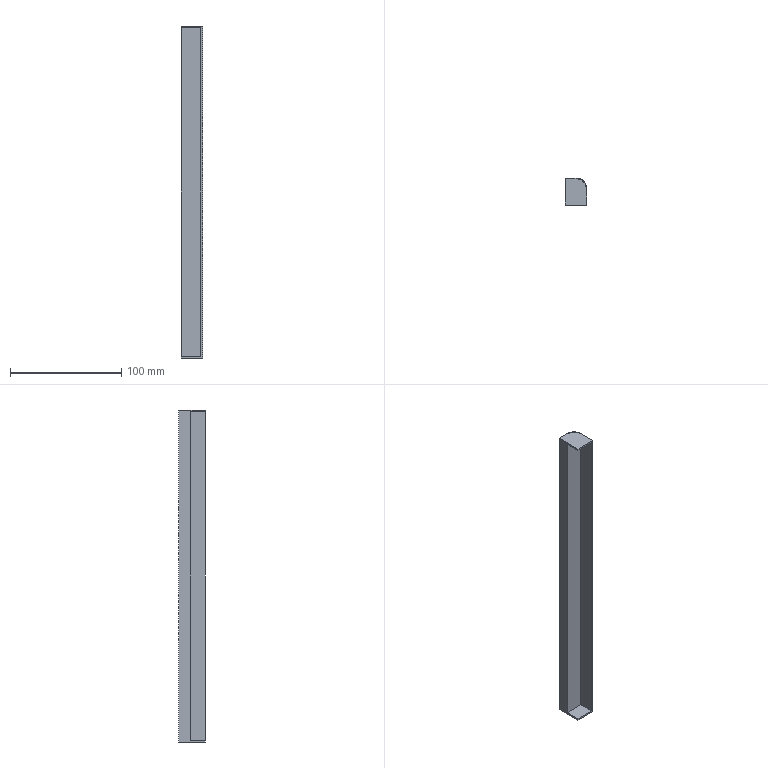Part | SolidWorks | features BaseBody 1 | 1 solid | 25 faces | box 19 x 24 x 298 mm | volume 61282 mm3 | cylinder 15 | plane 10 | commonest cylinder face diameters 1 x8 18 x7
STEP:
#1=CARTESIAN_POINT('',(17.2,0.,295.));
#2=VERTEX_POINT('',#1);
#3=CARTESIAN_POINT('',(17.2,0.,0.));
#4=VERTEX_POINT('',#3);
#5=CARTESIAN_POINT('',(17.2,0.,295.));
#6=DIRECTION('',(0.,0.,-1.));
#7=VECTOR('',#6,1000.);
#8=LINE('',#5,#7);
#9=EDGE_CURVE('',#2,#4,#8,.T.);
#10=ORIENTED_EDGE('',*,*,#9,.F.);
#11=CARTESIAN_POINT('',(0.,0.,295.));
#12=VERTEX_POINT('',#11);
#13=CARTESIAN_POINT('',(0.,0.,295.));
#14=DIRECTION('',(1.,0.,0.));
#15=VECTOR('',#14,1000.);
#16=LINE('',#13,#15);
#17=EDGE_CURVE('',#12,#2,#16,.T.);
#18=ORIENTED_EDGE('',*,*,#17,.F.);
#19=CARTESIAN_POINT('',(0.,0.,0.));
#20=VERTEX_POINT('',#19);
#21=CARTESIAN_POINT('',(0.,0.,295.));
#22=DIRECTION('',(0.,0.,1.));
#23=VECTOR('',#22,1000.);
#24=LINE('',#21,#23);
#25=EDGE_CURVE('',#20,#12,#24,.T.);
#26=ORIENTED_EDGE('',*,*,#25,.F.);
#27=CARTESIAN_POINT('',(0.,0.,0.));
#28=DIRECTION('',(-1.,0.,0.));
#29=VECTOR('',#28,1000.);
#30=LINE('',#27,#29);
#31=EDGE_CURVE('',#4,#20,#30,.T.);
#32=ORIENTED_EDGE('',*,*,#31,.F.);
#33=EDGE_LOOP('',(#10,#18,#26,#32));
#34=FACE_OUTER_BOUND('',#33,.T.);
#35=CARTESIAN_POINT('',(0.,0.,295.));
#36=DIRECTION('',(0.,1.,0.));
#37=DIRECTION('',(0.,0.,1.));
#38=AXIS2_PLACEMENT_3D('',#35,#36,#37);
#39=PLANE('',#38);
#40=ADVANCED_FACE('',(#34),#39,.F.);
#41=CARTESIAN_POINT('',(0.,-13.5,0.));
#42=VERTEX_POINT('',#41);
#43=CARTESIAN_POINT('',(0.,1.5,0.));
#44=DIRECTION('',(0.,1.,0.));
#45=VECTOR('',#44,1000.);
#46=LINE('',#43,#45);
#47=EDGE_CURVE('',#42,#20,#46,.T.);
#48=ORIENTED_EDGE('',*,*,#47,.F.);
#49=CARTESIAN_POINT('',(17.2,-13.5,0.));
#50=VERTEX_POINT('',#49);
#51=CARTESIAN_POINT('',(10.,-13.5,0.));
#52=DIRECTION('',(-1.,0.,0.));
#53=VECTOR('',#52,1000.);
#54=LINE('',#51,#53);
#55=EDGE_CURVE('',#50,#42,#54,.T.);
#56=ORIENTED_EDGE('',*,*,#55,.F.);
#57=CARTESIAN_POINT('',(17.2,1.5,0.));
#58=DIRECTION('',(0.,-1.,0.));
#59=VECTOR('',#58,1000.);
#60=LINE('',#57,#59);
#61=EDGE_CURVE('',#4,#50,#60,.T.);
#62=ORIENTED_EDGE('',*,*,#61,.F.);
#63=ORIENTED_EDGE('',*,*,#31,.T.);
#64=EDGE_LOOP('',(#48,#56,#62,#63));
#65=FACE_OUTER_BOUND('',#64,.T.);
#66=CARTESIAN_POINT('',(10.,1.5,0.));
#67=DIRECTION('',(0.,0.,-1.));
#68=DIRECTION('',(-1.,0.,0.));
#69=AXIS2_PLACEMENT_3D('',#66,#67,#68);
#70=PLANE('',#69);
#71=ADVANCED_FACE('',(#65),#70,.F.);
#72=CARTESIAN_POINT('',(17.2,-13.5,295.));
#73=VERTEX_POINT('',#72);
#74=CARTESIAN_POINT('',(17.2,-13.5,295.));
#75=DIRECTION('',(0.,0.,-1.));
#76=VECTOR('',#75,1000.);
#77=LINE('',#74,#76);
#78=EDGE_CURVE('',#73,#50,#77,.T.);
#79=ORIENTED_EDGE('',*,*,#78,.F.);
#80=CARTESIAN_POINT('',(17.2,0.,295.));
#81=DIRECTION('',(0.,-1.,0.));
#82=VECTOR('',#81,1000.);
#83=LINE('',#80,#82);
#84=EDGE_CURVE('',#2,#73,#83,.T.);
#85=ORIENTED_EDGE('',*,*,#84,.F.);
#86=ORIENTED_EDGE('',*,*,#9,.T.);
#87=ORIENTED_EDGE('',*,*,#61,.T.);
#88=EDGE_LOOP('',(#79,#85,#86,#87));
#89=FACE_OUTER_BOUND('',#88,.T.);
#90=CARTESIAN_POINT('',(17.2,0.,295.));
#91=DIRECTION('',(1.,0.,0.));
#92=DIRECTION('',(0.,0.,-1.));
#93=AXIS2_PLACEMENT_3D('',#90,#91,#92);
#94=PLANE('',#93);
#95=ADVANCED_FACE('',(#89),#94,.F.);
#96=ORIENTED_EDGE('',*,*,#17,.T.);
#97=ORIENTED_EDGE('',*,*,#84,.T.);
#98=CARTESIAN_POINT('',(0.,-13.5,295.));
#99=VERTEX_POINT('',#98);
#100=CARTESIAN_POINT('',(10.,-13.5,295.));
#101=DIRECTION('',(1.,0.,0.));
#102=VECTOR('',#101,1000.);
#103=LINE('',#100,#102);
#104=EDGE_CURVE('',#99,#73,#103,.T.);
#105=ORIENTED_EDGE('',*,*,#104,.F.);
#106=CARTESIAN_POINT('',(0.,1.5,295.));
#107=DIRECTION('',(0.,-1.,0.));
#108=VECTOR('',#107,1000.);
#109=LINE('',#106,#108);
#110=EDGE_CURVE('',#12,#99,#109,.T.);
#111=ORIENTED_EDGE('',*,*,#110,.F.);
#112=EDGE_LOOP('',(#96,#97,#105,#111));
#113=FACE_OUTER_BOUND('',#112,.T.);
#114=CARTESIAN_POINT('',(10.,1.5,295.));
#115=DIRECTION('',(0.,0.,1.));
#116=DIRECTION('',(1.,0.,0.));
#117=AXIS2_PLACEMENT_3D('',#114,#115,#116);
#118=PLANE('',#117);
#119=ADVANCED_FACE('',(#113),#118,.F.);
#120=CARTESIAN_POINT('',(0.,-13.5,-1.5));
#121=VERTEX_POINT('',#120);
#122=CARTESIAN_POINT('',(0.,10.5,-1.5));
#123=VERTEX_POINT('',#122);
#124=CARTESIAN_POINT('',(0.,0.,-1.5));
#125=DIRECTION('',(0.,1.,0.));
#126=VECTOR('',#125,1000.);
#127=LINE('',#124,#126);
#128=EDGE_CURVE('',#121,#123,#127,.T.);
#129=ORIENTED_EDGE('',*,*,#128,.F.);
#130=CARTESIAN_POINT('',(0.,-13.5,295.));
#131=DIRECTION('',(0.,0.,-1.));
#132=VECTOR('',#131,1000.);
#133=LINE('',#130,#132);
#134=EDGE_CURVE('',#42,#121,#133,.T.);
#135=ORIENTED_EDGE('',*,*,#134,.F.);
#136=ORIENTED_EDGE('',*,*,#47,.T.);
#137=ORIENTED_EDGE('',*,*,#25,.T.);
#138=ORIENTED_EDGE('',*,*,#110,.T.);
#139=CARTESIAN_POINT('',(0.,-13.5,296.5));
#140=VERTEX_POINT('',#139);
#141=CARTESIAN_POINT('',(0.,-13.5,295.));
#142=DIRECTION('',(0.,0.,-1.));
#143=VECTOR('',#142,1000.);
#144=LINE('',#141,#143);
#145=EDGE_CURVE('',#140,#99,#144,.T.);
#146=ORIENTED_EDGE('',*,*,#145,.F.);
#147=CARTESIAN_POINT('',(0.,10.5,296.5));
#148=VERTEX_POINT('',#147);
#149=CARTESIAN_POINT('',(0.,0.,296.5));
#150=DIRECTION('',(0.,-1.,0.));
#151=VECTOR('',#150,1000.);
#152=LINE('',#149,#151);
#153=EDGE_CURVE('',#148,#140,#152,.T.);
#154=ORIENTED_EDGE('',*,*,#153,.F.);
#155=CARTESIAN_POINT('',(0.,10.5,295.));
#156=DIRECTION('',(0.,0.,1.));
#157=VECTOR('',#156,1000.);
#158=LINE('',#155,#157);
#159=EDGE_CURVE('',#123,#148,#158,.T.);
#160=ORIENTED_EDGE('',*,*,#159,.F.);
#161=EDGE_LOOP('',(#129,#135,#136,#137,#138,#146,#154,#160));
#162=FACE_OUTER_BOUND('',#161,.T.);
#163=CARTESIAN_POINT('',(0.,0.,295.));
#164=DIRECTION('',(1.,0.,0.));
#165=DIRECTION('',(0.,0.,-1.));
#166=AXIS2_PLACEMENT_3D('',#163,#164,#165);
#167=PLANE('',#166);
#168=ADVANCED_FACE('',(#162),#167,.F.);
#169=ORIENTED_EDGE('',*,*,#55,.T.);
#170=ORIENTED_EDGE('',*,*,#134,.T.);
#171=CARTESIAN_POINT('',(19.,-13.5,-1.5));
#172=VERTEX_POINT('',#171);
#173=CARTESIAN_POINT('',(17.2,-13.5,-1.5));
#174=DIRECTION('',(-1.,0.,0.));
#175=VECTOR('',#174,1000.);
#176=LINE('',#173,#175);
#177=EDGE_CURVE('',#172,#121,#176,.T.);
#178=ORIENTED_EDGE('',*,*,#177,.F.);
#179=CARTESIAN_POINT('',(19.,-13.5,296.5));
#180=VERTEX_POINT('',#179);
#181=CARTESIAN_POINT('',(19.,-13.5,295.));
#182=DIRECTION('',(0.,0.,-1.));
#183=VECTOR('',#182,1000.);
#184=LINE('',#181,#183);
#185=EDGE_CURVE('',#180,#172,#184,.T.);
#186=ORIENTED_EDGE('',*,*,#185,.F.);
#187=CARTESIAN_POINT('',(17.2,-13.5,296.5));
#188=DIRECTION('',(1.,0.,0.));
#189=VECTOR('',#188,1000.);
#190=LINE('',#187,#189);
#191=EDGE_CURVE('',#140,#180,#190,.T.);
#192=ORIENTED_EDGE('',*,*,#191,.F.);
#193=ORIENTED_EDGE('',*,*,#145,.T.);
#194=ORIENTED_EDGE('',*,*,#104,.T.);
#195=ORIENTED_EDGE('',*,*,#78,.T.);
#196=EDGE_LOOP('',(#169,#170,#178,#186,#192,#193,#194,#195));
#197=FACE_OUTER_BOUND('',#196,.T.);
#198=CARTESIAN_POINT('',(17.2,-13.5,295.));
#199=DIRECTION('',(0.,1.,0.));
#200=DIRECTION('',(0.,0.,1.));
#201=AXIS2_PLACEMENT_3D('',#198,#199,#200);
#202=PLANE('',#201);
#203=ADVANCED_FACE('',(#197),#202,.F.);
#204=CARTESIAN_POINT('',(9.5,10.5,-1.5));
#205=VERTEX_POINT('',#204);
#206=CARTESIAN_POINT('',(9.5,10.5,296.5));
#207=VERTEX_POINT('',#206);
#208=CARTESIAN_POINT('',(9.5,10.5,295.));
#209=DIRECTION('',(0.,0.,1.));
#210=VECTOR('',#209,1000.);
#211=LINE('',#208,#210);
#212=EDGE_CURVE('',#205,#207,#211,.T.);
#213=ORIENTED_EDGE('',*,*,#212,.F.);
#214=CARTESIAN_POINT('',(0.,10.5,-1.5));
#215=DIRECTION('',(1.,0.,0.));
#216=VECTOR('',#215,1000.);
#217=LINE('',#214,#216);
#218=EDGE_CURVE('',#123,#205,#217,.T.);
#219=ORIENTED_EDGE('',*,*,#218,.F.);
#220=ORIENTED_EDGE('',*,*,#159,.T.);
#221=CARTESIAN_POINT('',(0.,10.5,296.5));
#222=DIRECTION('',(-1.,0.,0.));
#223=VECTOR('',#222,1000.);
#224=LINE('',#221,#223);
#225=EDGE_CURVE('',#207,#148,#224,.T.);
#226=ORIENTED_EDGE('',*,*,#225,.F.);
#227=EDGE_LOOP('',(#213,#219,#220,#226));
#228=FACE_OUTER_BOUND('',#227,.T.);
#229=CARTESIAN_POINT('',(0.,10.5,295.));
#230=DIRECTION('',(0.,-1.,0.));
#231=DIRECTION('',(0.,0.,-1.));
#232=AXIS2_PLACEMENT_3D('',#229,#230,#231);
#233=PLANE('',#232);
#234=ADVANCED_FACE('',(#228),#233,.F.);
#235=ORIENTED_EDGE('',*,*,#128,.T.);
#236=ORIENTED_EDGE('',*,*,#218,.T.);
#237=CARTESIAN_POINT('',(10.5,10.486,-1.5));
#238=VERTEX_POINT('',#237);
#239=CARTESIAN_POINT('',(10.,10.5,-1.5));
#240=DIRECTION('',(0.,0.,1.));
#241=DIRECTION('',(1.,0.,0.));
#242=AXIS2_PLACEMENT_3D('',#239,#240,#241);
#243=CIRCLE('',#242,0.5);
#244=EDGE_CURVE('',#205,#238,#243,.T.);
#245=ORIENTED_EDGE('',*,*,#244,.T.);
#246=CARTESIAN_POINT('',(11.512,10.372,-1.5));
#247=VERTEX_POINT('',#246);
#248=CARTESIAN_POINT('',(10.,1.5,-1.5));
#249=DIRECTION('',(0.,0.,1.));
#250=DIRECTION('',(-1.,0.,0.));
#251=AXIS2_PLACEMENT_3D('',#248,#249,#250);
#252=CIRCLE('',#251,9.);
#253=EDGE_CURVE('',#247,#238,#252,.T.);
#254=ORIENTED_EDGE('',*,*,#253,.F.);
#255=CARTESIAN_POINT('',(12.487,10.15,-1.5));
#256=VERTEX_POINT('',#255);
#257=CARTESIAN_POINT('',(12.003,10.274,-1.5));
#258=DIRECTION('',(0.,0.,1.));
#259=DIRECTION('',(1.,0.,0.));
#260=AXIS2_PLACEMENT_3D('',#257,#258,#259);
#261=CIRCLE('',#260,0.5);
#262=EDGE_CURVE('',#247,#256,#261,.T.);
#263=ORIENTED_EDGE('',*,*,#262,.T.);
#264=CARTESIAN_POINT('',(13.449,9.813,-1.5));
#265=VERTEX_POINT('',#264);
#266=CARTESIAN_POINT('',(10.,1.5,-1.5));
#267=DIRECTION('',(0.,0.,1.));
#268=DIRECTION('',(-1.,0.,0.));
#269=AXIS2_PLACEMENT_3D('',#266,#267,#268);
#270=CIRCLE('',#269,9.);
#271=EDGE_CURVE('',#265,#256,#270,.T.);
#272=ORIENTED_EDGE('',*,*,#271,.F.);
#273=CARTESIAN_POINT('',(14.349,9.379,-1.5));
#274=VERTEX_POINT('',#273);
#275=CARTESIAN_POINT('',(13.905,9.609,-1.5));
#276=DIRECTION('',(0.,0.,1.));
#277=DIRECTION('',(1.,0.,0.));
#278=AXIS2_PLACEMENT_3D('',#275,#276,#277);
#279=CIRCLE('',#278,0.5);
#280=EDGE_CURVE('',#265,#274,#279,.T.);
#281=ORIENTED_EDGE('',*,*,#280,.T.);
#282=CARTESIAN_POINT('',(15.212,8.837,-1.5));
#283=VERTEX_POINT('',#282);
#284=CARTESIAN_POINT('',(10.,1.5,-1.5));
#285=DIRECTION('',(0.,0.,1.));
#286=DIRECTION('',(-1.,0.,0.));
#287=AXIS2_PLACEMENT_3D('',#284,#285,#286);
#288=CIRCLE('',#287,9.);
#289=EDGE_CURVE('',#283,#274,#288,.T.);
#290=ORIENTED_EDGE('',*,*,#289,.F.);
#291=CARTESIAN_POINT('',(15.994,8.214,-1.5));
#292=VERTEX_POINT('',#291);
#293=CARTESIAN_POINT('',(15.611,8.536,-1.5));
#294=DIRECTION('',(0.,0.,1.));
#295=DIRECTION('',(1.,0.,0.));
#296=AXIS2_PLACEMENT_3D('',#293,#294,#295);
#297=CIRCLE('',#296,0.5);
#298=EDGE_CURVE('',#283,#292,#297,.T.);
#299=ORIENTED_EDGE('',*,*,#298,.T.);
#300=CARTESIAN_POINT('',(16.714,7.494,-1.5));
#301=VERTEX_POINT('',#300);
#302=CARTESIAN_POINT('',(10.,1.5,-1.5));
#303=DIRECTION('',(0.,0.,1.));
#304=DIRECTION('',(-1.,0.,0.));
#305=AXIS2_PLACEMENT_3D('',#302,#303,#304);
#306=CIRCLE('',#305,9.);
#307=EDGE_CURVE('',#301,#292,#306,.T.);
#308=ORIENTED_EDGE('',*,*,#307,.F.);
#309=CARTESIAN_POINT('',(17.337,6.712,-1.5));
#310=VERTEX_POINT('',#309);
#311=CARTESIAN_POINT('',(17.036,7.111,-1.5));
#312=DIRECTION('',(0.,0.,1.));
#313=DIRECTION('',(1.,0.,0.));
#314=AXIS2_PLACEMENT_3D('',#311,#312,#313);
#315=CIRCLE('',#314,0.5);
#316=EDGE_CURVE('',#301,#310,#315,.T.);
#317=ORIENTED_EDGE('',*,*,#316,.T.);
#318=CARTESIAN_POINT('',(17.879,5.849,-1.5));
#319=VERTEX_POINT('',#318);
#320=CARTESIAN_POINT('',(10.,1.5,-1.5));
#321=DIRECTION('',(0.,0.,1.));
#322=DIRECTION('',(-1.,0.,0.));
#323=AXIS2_PLACEMENT_3D('',#320,#321,#322);
#324=CIRCLE('',#323,9.);
#325=EDGE_CURVE('',#319,#310,#324,.T.);
#326=ORIENTED_EDGE('',*,*,#325,.F.);
#327=CARTESIAN_POINT('',(18.313,4.949,-1.5));
#328=VERTEX_POINT('',#327);
#329=CARTESIAN_POINT('',(18.109,5.405,-1.5));
#330=DIRECTION('',(0.,0.,1.));
#331=DIRECTION('',(1.,0.,0.));
#332=AXIS2_PLACEMENT_3D('',#329,#330,#331);
#333=CIRCLE('',#332,0.5);
#334=EDGE_CURVE('',#319,#328,#333,.T.);
#335=ORIENTED_EDGE('',*,*,#334,.T.);
#336=CARTESIAN_POINT('',(18.65,3.987,-1.5));
#337=VERTEX_POINT('',#336);
#338=CARTESIAN_POINT('',(10.,1.5,-1.5));
#339=DIRECTION('',(0.,0.,1.));
#340=DIRECTION('',(-1.,0.,0.));
#341=AXIS2_PLACEMENT_3D('',#338,#339,#340);
#342=CIRCLE('',#341,9.);
#343=EDGE_CURVE('',#337,#328,#342,.T.);
#344=ORIENTED_EDGE('',*,*,#343,.F.);
#345=CARTESIAN_POINT('',(18.872,3.012,-1.5));
#346=VERTEX_POINT('',#345);
#347=CARTESIAN_POINT('',(18.774,3.503,-1.5));
#348=DIRECTION('',(0.,0.,1.));
#349=DIRECTION('',(1.,0.,0.));
#350=AXIS2_PLACEMENT_3D('',#347,#348,#349);
#351=CIRCLE('',#350,0.5);
#352=EDGE_CURVE('',#337,#346,#351,.T.);
#353=ORIENTED_EDGE('',*,*,#352,.T.);
#354=CARTESIAN_POINT('',(18.986,2.,-1.5));
#355=VERTEX_POINT('',#354);
#356=CARTESIAN_POINT('',(10.,1.5,-1.5));
#357=DIRECTION('',(0.,0.,1.));
#358=DIRECTION('',(-1.,0.,0.));
#359=AXIS2_PLACEMENT_3D('',#356,#357,#358);
#360=CIRCLE('',#359,9.);
#361=EDGE_CURVE('',#355,#346,#360,.T.);
#362=ORIENTED_EDGE('',*,*,#361,.F.);
#363=CARTESIAN_POINT('',(19.,1.,-1.5));
#364=VERTEX_POINT('',#363);
#365=CARTESIAN_POINT('',(19.,1.5,-1.5));
#366=DIRECTION('',(0.,0.,1.));
#367=DIRECTION('',(1.,0.,0.));
#368=AXIS2_PLACEMENT_3D('',#365,#366,#367);
#369=CIRCLE('',#368,0.5);
#370=EDGE_CURVE('',#355,#364,#369,.T.);
#371=ORIENTED_EDGE('',*,*,#370,.T.);
#372=CARTESIAN_POINT('',(19.,1.5,-1.5));
#373=DIRECTION('',(0.,-1.,0.));
#374=VECTOR('',#373,1000.);
#375=LINE('',#372,#374);
#376=EDGE_CURVE('',#364,#172,#375,.T.);
#377=ORIENTED_EDGE('',*,*,#376,.T.);
#378=ORIENTED_EDGE('',*,*,#177,.T.);
#379=EDGE_LOOP('',(#235,#236,#245,#254,#263,#272,#281,#290,#299,#308,#317,#326,#335,#344,#353,#362,#371,#377,#378));
#380=FACE_OUTER_BOUND('',#379,.T.);
#381=CARTESIAN_POINT('',(10.,1.5,-1.5));
#382=DIRECTION('',(0.,0.,-1.));
#383=DIRECTION('',(-1.,0.,0.));
#384=AXIS2_PLACEMENT_3D('',#381,#382,#383);
#385=PLANE('',#384);
#386=ADVANCED_FACE('',(#380),#385,.T.);
#387=CARTESIAN_POINT('',(12.487,10.15,296.5));
#388=VERTEX_POINT('',#387);
#389=CARTESIAN_POINT('',(11.512,10.372,296.5));
#390=VERTEX_POINT('',#389);
#391=CARTESIAN_POINT('',(12.003,10.274,296.5));
#392=DIRECTION('',(0.,0.,-1.));
#393=DIRECTION('',(1.,0.,0.));
#394=AXIS2_PLACEMENT_3D('',#391,#392,#393);
#395=CIRCLE('',#394,0.5);
#396=EDGE_CURVE('',#388,#390,#395,.T.);
#397=ORIENTED_EDGE('',*,*,#396,.T.);
#398=CARTESIAN_POINT('',(10.5,10.486,296.5));
#399=VERTEX_POINT('',#398);
#400=CARTESIAN_POINT('',(10.,1.5,296.5));
#401=DIRECTION('',(0.,0.,-1.));
#402=DIRECTION('',(-1.,0.,0.));
#403=AXIS2_PLACEMENT_3D('',#400,#401,#402);
#404=CIRCLE('',#403,9.);
#405=EDGE_CURVE('',#399,#390,#404,.T.);
#406=ORIENTED_EDGE('',*,*,#405,.F.);
#407=CARTESIAN_POINT('',(10.,10.5,296.5));
#408=DIRECTION('',(0.,0.,-1.));
#409=DIRECTION('',(1.,0.,0.));
#410=AXIS2_PLACEMENT_3D('',#407,#408,#409);
#411=CIRCLE('',#410,0.5);
#412=EDGE_CURVE('',#399,#207,#411,.T.);
#413=ORIENTED_EDGE('',*,*,#412,.T.);
#414=ORIENTED_EDGE('',*,*,#225,.T.);
#415=ORIENTED_EDGE('',*,*,#153,.T.);
#416=ORIENTED_EDGE('',*,*,#191,.T.);
#417=CARTESIAN_POINT('',(19.,1.,296.5));
#418=VERTEX_POINT('',#417);
#419=CARTESIAN_POINT('',(19.,1.5,296.5));
#420=DIRECTION('',(0.,1.,0.));
#421=VECTOR('',#420,1000.);
#422=LINE('',#419,#421);
#423=EDGE_CURVE('',#180,#418,#422,.T.);
#424=ORIENTED_EDGE('',*,*,#423,.T.);
#425=CARTESIAN_POINT('',(18.986,2.,296.5));
#426=VERTEX_POINT('',#425);
#427=CARTESIAN_POINT('',(19.,1.5,296.5));
#428=DIRECTION('',(0.,0.,-1.));
#429=DIRECTION('',(1.,0.,0.));
#430=AXIS2_PLACEMENT_3D('',#427,#428,#429);
#431=CIRCLE('',#430,0.5);
#432=EDGE_CURVE('',#418,#426,#431,.T.);
#433=ORIENTED_EDGE('',*,*,#432,.T.);
#434=CARTESIAN_POINT('',(18.872,3.012,296.5));
#435=VERTEX_POINT('',#434);
#436=CARTESIAN_POINT('',(10.,1.5,296.5));
#437=DIRECTION('',(0.,0.,-1.));
#438=DIRECTION('',(-1.,0.,0.));
#439=AXIS2_PLACEMENT_3D('',#436,#437,#438);
#440=CIRCLE('',#439,9.);
#441=EDGE_CURVE('',#435,#426,#440,.T.);
#442=ORIENTED_EDGE('',*,*,#441,.F.);
#443=CARTESIAN_POINT('',(18.65,3.987,296.5));
#444=VERTEX_POINT('',#443);
#445=CARTESIAN_POINT('',(18.774,3.503,296.5));
#446=DIRECTION('',(0.,0.,-1.));
#447=DIRECTION('',(1.,0.,0.));
#448=AXIS2_PLACEMENT_3D('',#445,#446,#447);
#449=CIRCLE('',#448,0.5);
#450=EDGE_CURVE('',#435,#444,#449,.T.);
#451=ORIENTED_EDGE('',*,*,#450,.T.);
#452=CARTESIAN_POINT('',(18.313,4.949,296.5));
#453=VERTEX_POINT('',#452);
#454=CARTESIAN_POINT('',(10.,1.5,296.5));
#455=DIRECTION('',(0.,0.,-1.));
#456=DIRECTION('',(-1.,0.,0.));
#457=AXIS2_PLACEMENT_3D('',#454,#455,#456);
#458=CIRCLE('',#457,9.);
#459=EDGE_CURVE('',#453,#444,#458,.T.);
#460=ORIENTED_EDGE('',*,*,#459,.F.);
#461=CARTESIAN_POINT('',(17.879,5.849,296.5));
#462=VERTEX_POINT('',#461);
#463=CARTESIAN_POINT('',(18.109,5.405,296.5));
#464=DIRECTION('',(0.,0.,-1.));
#465=DIRECTION('',(1.,0.,0.));
#466=AXIS2_PLACEMENT_3D('',#463,#464,#465);
#467=CIRCLE('',#466,0.5);
#468=EDGE_CURVE('',#453,#462,#467,.T.);
#469=ORIENTED_EDGE('',*,*,#468,.T.);
#470=CARTESIAN_POINT('',(17.337,6.712,296.5));
#471=VERTEX_POINT('',#470);
#472=CARTESIAN_POINT('',(10.,1.5,296.5));
#473=DIRECTION('',(0.,0.,-1.));
#474=DIRECTION('',(-1.,0.,0.));
#475=AXIS2_PLACEMENT_3D('',#472,#473,#474);
#476=CIRCLE('',#475,9.);
#477=EDGE_CURVE('',#471,#462,#476,.T.);
#478=ORIENTED_EDGE('',*,*,#477,.F.);
#479=CARTESIAN_POINT('',(16.714,7.494,296.5));
#480=VERTEX_POINT('',#479);
#481=CARTESIAN_POINT('',(17.036,7.111,296.5));
#482=DIRECTION('',(0.,0.,-1.));
#483=DIRECTION('',(1.,0.,0.));
#484=AXIS2_PLACEMENT_3D('',#481,#482,#483);
#485=CIRCLE('',#484,0.5);
#486=EDGE_CURVE('',#471,#480,#485,.T.);
#487=ORIENTED_EDGE('',*,*,#486,.T.);
#488=CARTESIAN_POINT('',(15.994,8.214,296.5));
#489=VERTEX_POINT('',#488);
#490=CARTESIAN_POINT('',(10.,1.5,296.5));
#491=DIRECTION('',(0.,0.,-1.));
#492=DIRECTION('',(-1.,0.,0.));
#493=AXIS2_PLACEMENT_3D('',#490,#491,#492);
#494=CIRCLE('',#493,9.);
#495=EDGE_CURVE('',#489,#480,#494,.T.);
#496=ORIENTED_EDGE('',*,*,#495,.F.);
#497=CARTESIAN_POINT('',(15.212,8.837,296.5));
#498=VERTEX_POINT('',#497);
#499=CARTESIAN_POINT('',(15.611,8.536,296.5));
#500=DIRECTION('',(0.,0.,-1.));
#501=DIRECTION('',(1.,0.,0.));
#502=AXIS2_PLACEMENT_3D('',#499,#500,#501);
#503=CIRCLE('',#502,0.5);
#504=EDGE_CURVE('',#489,#498,#503,.T.);
#505=ORIENTED_EDGE('',*,*,#504,.T.);
#506=CARTESIAN_POINT('',(14.349,9.379,296.5));
#507=VERTEX_POINT('',#506);
#508=CARTESIAN_POINT('',(10.,1.5,296.5));
#509=DIRECTION('',(0.,0.,-1.));
#510=DIRECTION('',(-1.,0.,0.));
#511=AXIS2_PLACEMENT_3D('',#508,#509,#510);
#512=CIRCLE('',#511,9.);
#513=EDGE_CURVE('',#507,#498,#512,.T.);
#514=ORIENTED_EDGE('',*,*,#513,.F.);
#515=CARTESIAN_POINT('',(13.449,9.813,296.5));
#516=VERTEX_POINT('',#515);
#517=CARTESIAN_POINT('',(13.905,9.609,296.5));
#518=DIRECTION('',(0.,0.,-1.));
#519=DIRECTION('',(1.,0.,0.));
#520=AXIS2_PLACEMENT_3D('',#517,#518,#519);
#521=CIRCLE('',#520,0.5);
#522=EDGE_CURVE('',#507,#516,#521,.T.);
#523=ORIENTED_EDGE('',*,*,#522,.T.);
#524=CARTESIAN_POINT('',(10.,1.5,296.5));
#525=DIRECTION('',(0.,0.,-1.));
#526=DIRECTION('',(-1.,0.,0.));
#527=AXIS2_PLACEMENT_3D('',#524,#525,#526);
#528=CIRCLE('',#527,9.);
#529=EDGE_CURVE('',#388,#516,#528,.T.);
#530=ORIENTED_EDGE('',*,*,#529,.F.);
#531=EDGE_LOOP('',(#397,#406,#413,#414,#415,#416,#424,#433,#442,#451,#460,#469,#478,#487,#496,#505,#514,#523,#530));
#532=FACE_OUTER_BOUND('',#531,.T.);
#533=CARTESIAN_POINT('',(10.,1.5,296.5));
#534=DIRECTION('',(0.,0.,1.));
#535=DIRECTION('',(1.,0.,0.));
#536=AXIS2_PLACEMENT_3D('',#533,#534,#535);
#537=PLANE('',#536);
#538=ADVANCED_FACE('',(#532),#537,.T.);
#539=CARTESIAN_POINT('',(19.,1.,295.));
#540=DIRECTION('',(0.,0.,-1.));
#541=VECTOR('',#540,1000.);
#542=LINE('',#539,#541);
#543=EDGE_CURVE('',#418,#364,#542,.T.);
#544=ORIENTED_EDGE('',*,*,#543,.F.);
#545=ORIENTED_EDGE('',*,*,#423,.F.);
#546=ORIENTED_EDGE('',*,*,#185,.T.);
#547=ORIENTED_EDGE('',*,*,#376,.F.);
#548=EDGE_LOOP('',(#544,#545,#546,#547));
#549=FACE_OUTER_BOUND('',#548,.T.);
#550=CARTESIAN_POINT('',(19.,1.5,295.));
#551=DIRECTION('',(-1.,0.,0.));
#552=DIRECTION('',(0.,-1.,0.));
#553=AXIS2_PLACEMENT_3D('',#550,#551,#552);
#554=PLANE('',#553);
#555=ADVANCED_FACE('',(#549),#554,.F.);
#556=ORIENTED_EDGE('',*,*,#212,.T.);
#557=ORIENTED_EDGE('',*,*,#412,.F.);
#558=CARTESIAN_POINT('',(10.5,10.486,-1.5));
#559=DIRECTION('',(0.,0.,1.));
#560=VECTOR('',#559,1000.);
#561=LINE('',#558,#560);
#562=EDGE_CURVE('',#238,#399,#561,.T.);
#563=ORIENTED_EDGE('',*,*,#562,.F.);
#564=ORIENTED_EDGE('',*,*,#244,.F.);
#565=EDGE_LOOP('',(#556,#557,#563,#564));
#566=FACE_OUTER_BOUND('',#565,.T.);
#567=CARTESIAN_POINT('',(10.,10.5,-1.5));
#568=DIRECTION('',(0.,0.,1.));
#569=DIRECTION('',(1.,0.,0.));
#570=AXIS2_PLACEMENT_3D('',#567,#568,#569);
#571=CYLINDRICAL_SURFACE('',#570,0.5);
#572=ADVANCED_FACE('',(#566),#571,.F.);
#573=CARTESIAN_POINT('',(18.986,2.,-1.5));
#574=DIRECTION('',(0.,0.,-1.));
#575=VECTOR('',#574,1000.);
#576=LINE('',#573,#575);
#577=EDGE_CURVE('',#426,#355,#576,.T.);
#578=ORIENTED_EDGE('',*,*,#577,.F.);
#579=ORIENTED_EDGE('',*,*,#432,.F.);
#580=ORIENTED_EDGE('',*,*,#543,.T.);
#581=ORIENTED_EDGE('',*,*,#370,.F.);
#582=EDGE_LOOP('',(#578,#579,#580,#581));
#583=FACE_OUTER_BOUND('',#582,.T.);
#584=CARTESIAN_POINT('',(19.,1.5,-1.5));
#585=DIRECTION('',(0.,0.,1.));
#586=DIRECTION('',(1.,0.,0.));
#587=AXIS2_PLACEMENT_3D('',#584,#585,#586);
#588=CYLINDRICAL_SURFACE('',#587,0.5);
#589=ADVANCED_FACE('',(#583),#588,.F.);
#590=ORIENTED_EDGE('',*,*,#405,.T.);
#591=CARTESIAN_POINT('',(11.512,10.372,295.));
#592=DIRECTION('',(0.,0.,-1.));
#593=VECTOR('',#592,1000.);
#594=LINE('',#591,#593);
#595=EDGE_CURVE('',#390,#247,#594,.T.);
#596=ORIENTED_EDGE('',*,*,#595,.T.);
#597=ORIENTED_EDGE('',*,*,#253,.T.);
#598=ORIENTED_EDGE('',*,*,#562,.T.);
#599=EDGE_LOOP('',(#590,#596,#597,#598));
#600=FACE_OUTER_BOUND('',#599,.T.);
#601=CARTESIAN_POINT('',(10.,1.5,295.));
#602=DIRECTION('',(0.,0.,-1.));
#603=DIRECTION('',(-1.,0.,0.));
#604=AXIS2_PLACEMENT_3D('',#601,#602,#603);
#605=CYLINDRICAL_SURFACE('',#604,9.);
#606=ADVANCED_FACE('',(#600),#605,.T.);
#607=ORIENTED_EDGE('',*,*,#441,.T.);
#608=ORIENTED_EDGE('',*,*,#577,.T.);
#609=ORIENTED_EDGE('',*,*,#361,.T.);
#610=CARTESIAN_POINT('',(18.872,3.012,295.));
#611=DIRECTION('',(0.,0.,1.));
#612=VECTOR('',#611,1000.);
#613=LINE('',#610,#612);
#614=EDGE_CURVE('',#346,#435,#613,.T.);
#615=ORIENTED_EDGE('',*,*,#614,.T.);
#616=EDGE_LOOP('',(#607,#608,#609,#615));
#617=FACE_OUTER_BOUND('',#616,.T.);
#618=CARTESIAN_POINT('',(10.,1.5,295.));
#619=DIRECTION('',(0.,0.,-1.));
#620=DIRECTION('',(-1.,0.,0.));
#621=AXIS2_PLACEMENT_3D('',#618,#619,#620);
#622=CYLINDRICAL_SURFACE('',#621,9.);
#623=ADVANCED_FACE('',(#617),#622,.T.);
#624=ORIENTED_EDGE('',*,*,#595,.F.);
#625=ORIENTED_EDGE('',*,*,#396,.F.);
#626=CARTESIAN_POINT('',(12.487,10.15,-1.5));
#627=DIRECTION('',(0.,0.,1.));
#628=VECTOR('',#627,1000.);
#629=LINE('',#626,#628);
#630=EDGE_CURVE('',#256,#388,#629,.T.);
#631=ORIENTED_EDGE('',*,*,#630,.F.);
#632=ORIENTED_EDGE('',*,*,#262,.F.);
#633=EDGE_LOOP('',(#624,#625,#631,#632));
#634=FACE_OUTER_BOUND('',#633,.T.);
#635=CARTESIAN_POINT('',(12.003,10.274,-1.5));
#636=DIRECTION('',(0.,0.,1.));
#637=DIRECTION('',(1.,0.,0.));
#638=AXIS2_PLACEMENT_3D('',#635,#636,#637);
#639=CYLINDRICAL_SURFACE('',#638,0.5);
#640=ADVANCED_FACE('',(#634),#639,.F.);
#641=CARTESIAN_POINT('',(18.65,3.987,-1.5));
#642=DIRECTION('',(0.,0.,-1.));
#643=VECTOR('',#642,1000.);
#644=LINE('',#641,#643);
#645=EDGE_CURVE('',#444,#337,#644,.T.);
#646=ORIENTED_EDGE('',*,*,#645,.F.);
#647=ORIENTED_EDGE('',*,*,#450,.F.);
#648=ORIENTED_EDGE('',*,*,#614,.F.);
#649=ORIENTED_EDGE('',*,*,#352,.F.);
#650=EDGE_LOOP('',(#646,#647,#648,#649));
#651=FACE_OUTER_BOUND('',#650,.T.);
#652=CARTESIAN_POINT('',(18.774,3.503,-1.5));
#653=DIRECTION('',(0.,0.,1.));
#654=DIRECTION('',(1.,0.,0.));
#655=AXIS2_PLACEMENT_3D('',#652,#653,#654);
#656=CYLINDRICAL_SURFACE('',#655,0.5);
#657=ADVANCED_FACE('',(#651),#656,.F.);
#658=ORIENTED_EDGE('',*,*,#529,.T.);
#659=CARTESIAN_POINT('',(13.449,9.813,295.));
#660=DIRECTION('',(0.,0.,-1.));
#661=VECTOR('',#660,1000.);
#662=LINE('',#659,#661);
#663=EDGE_CURVE('',#516,#265,#662,.T.);
#664=ORIENTED_EDGE('',*,*,#663,.T.);
#665=ORIENTED_EDGE('',*,*,#271,.T.);
#666=ORIENTED_EDGE('',*,*,#630,.T.);
#667=EDGE_LOOP('',(#658,#664,#665,#666));
#668=FACE_OUTER_BOUND('',#667,.T.);
#669=CARTESIAN_POINT('',(10.,1.5,295.));
#670=DIRECTION('',(0.,0.,-1.));
#671=DIRECTION('',(-1.,0.,0.));
#672=AXIS2_PLACEMENT_3D('',#669,#670,#671);
#673=CYLINDRICAL_SURFACE('',#672,9.);
#674=ADVANCED_FACE('',(#668),#673,.T.);
#675=ORIENTED_EDGE('',*,*,#459,.T.);
#676=ORIENTED_EDGE('',*,*,#645,.T.);
#677=ORIENTED_EDGE('',*,*,#343,.T.);
#678=CARTESIAN_POINT('',(18.313,4.949,295.));
#679=DIRECTION('',(0.,0.,1.));
#680=VECTOR('',#679,1000.);
#681=LINE('',#678,#680);
#682=EDGE_CURVE('',#328,#453,#681,.T.);
#683=ORIENTED_EDGE('',*,*,#682,.T.);
#684=EDGE_LOOP('',(#675,#676,#677,#683));
#685=FACE_OUTER_BOUND('',#684,.T.);
#686=CARTESIAN_POINT('',(10.,1.5,295.));
#687=DIRECTION('',(0.,0.,-1.));
#688=DIRECTION('',(-1.,0.,0.));
#689=AXIS2_PLACEMENT_3D('',#686,#687,#688);
#690=CYLINDRICAL_SURFACE('',#689,9.);
#691=ADVANCED_FACE('',(#685),#690,.T.);
#692=ORIENTED_EDGE('',*,*,#663,.F.);
#693=ORIENTED_EDGE('',*,*,#522,.F.);
#694=CARTESIAN_POINT('',(14.349,9.379,-1.5));
#695=DIRECTION('',(0.,0.,1.));
#696=VECTOR('',#695,1000.);
#697=LINE('',#694,#696);
#698=EDGE_CURVE('',#274,#507,#697,.T.);
#699=ORIENTED_EDGE('',*,*,#698,.F.);
#700=ORIENTED_EDGE('',*,*,#280,.F.);
#701=EDGE_LOOP('',(#692,#693,#699,#700));
#702=FACE_OUTER_BOUND('',#701,.T.);
#703=CARTESIAN_POINT('',(13.905,9.609,-1.5));
#704=DIRECTION('',(0.,0.,1.));
#705=DIRECTION('',(1.,0.,0.));
#706=AXIS2_PLACEMENT_3D('',#703,#704,#705);
#707=CYLINDRICAL_SURFACE('',#706,0.5);
#708=ADVANCED_FACE('',(#702),#707,.F.);
#709=CARTESIAN_POINT('',(17.879,5.849,-1.5));
#710=DIRECTION('',(0.,0.,-1.));
#711=VECTOR('',#710,1000.);
#712=LINE('',#709,#711);
#713=EDGE_CURVE('',#462,#319,#712,.T.);
#714=ORIENTED_EDGE('',*,*,#713,.F.);
#715=ORIENTED_EDGE('',*,*,#468,.F.);
#716=ORIENTED_EDGE('',*,*,#682,.F.);
#717=ORIENTED_EDGE('',*,*,#334,.F.);
#718=EDGE_LOOP('',(#714,#715,#716,#717));
#719=FACE_OUTER_BOUND('',#718,.T.);
#720=CARTESIAN_POINT('',(18.109,5.405,-1.5));
#721=DIRECTION('',(0.,0.,1.));
#722=DIRECTION('',(1.,0.,0.));
#723=AXIS2_PLACEMENT_3D('',#720,#721,#722);
#724=CYLINDRICAL_SURFACE('',#723,0.5);
#725=ADVANCED_FACE('',(#719),#724,.F.);
#726=ORIENTED_EDGE('',*,*,#513,.T.);
#727=CARTESIAN_POINT('',(15.212,8.837,295.));
#728=DIRECTION('',(0.,0.,-1.));
#729=VECTOR('',#728,1000.);
#730=LINE('',#727,#729);
#731=EDGE_CURVE('',#498,#283,#730,.T.);
#732=ORIENTED_EDGE('',*,*,#731,.T.);
#733=ORIENTED_EDGE('',*,*,#289,.T.);
#734=ORIENTED_EDGE('',*,*,#698,.T.);
#735=EDGE_LOOP('',(#726,#732,#733,#734));
#736=FACE_OUTER_BOUND('',#735,.T.);
#737=CARTESIAN_POINT('',(10.,1.5,295.));
#738=DIRECTION('',(0.,0.,-1.));
#739=DIRECTION('',(-1.,0.,0.));
#740=AXIS2_PLACEMENT_3D('',#737,#738,#739);
#741=CYLINDRICAL_SURFACE('',#740,9.);
#742=ADVANCED_FACE('',(#736),#741,.T.);
#743=ORIENTED_EDGE('',*,*,#477,.T.);
#744=ORIENTED_EDGE('',*,*,#713,.T.);
#745=ORIENTED_EDGE('',*,*,#325,.T.);
#746=CARTESIAN_POINT('',(17.337,6.712,295.));
#747=DIRECTION('',(0.,0.,1.));
#748=VECTOR('',#747,1000.);
#749=LINE('',#746,#748);
#750=EDGE_CURVE('',#310,#471,#749,.T.);
#751=ORIENTED_EDGE('',*,*,#750,.T.);
#752=EDGE_LOOP('',(#743,#744,#745,#751));
#753=FACE_OUTER_BOUND('',#752,.T.);
#754=CARTESIAN_POINT('',(10.,1.5,295.));
#755=DIRECTION('',(0.,0.,-1.));
#756=DIRECTION('',(-1.,0.,0.));
#757=AXIS2_PLACEMENT_3D('',#754,#755,#756);
#758=CYLINDRICAL_SURFACE('',#757,9.);
#759=ADVANCED_FACE('',(#753),#758,.T.);
#760=ORIENTED_EDGE('',*,*,#731,.F.);
#761=ORIENTED_EDGE('',*,*,#504,.F.);
#762=CARTESIAN_POINT('',(15.994,8.214,-1.5));
#763=DIRECTION('',(0.,0.,1.));
#764=VECTOR('',#763,1000.);
#765=LINE('',#762,#764);
#766=EDGE_CURVE('',#292,#489,#765,.T.);
#767=ORIENTED_EDGE('',*,*,#766,.F.);
#768=ORIENTED_EDGE('',*,*,#298,.F.);
#769=EDGE_LOOP('',(#760,#761,#767,#768));
#770=FACE_OUTER_BOUND('',#769,.T.);
#771=CARTESIAN_POINT('',(15.611,8.536,-1.5));
#772=DIRECTION('',(0.,0.,1.));
#773=DIRECTION('',(1.,0.,0.));
#774=AXIS2_PLACEMENT_3D('',#771,#772,#773);
#775=CYLINDRICAL_SURFACE('',#774,0.5);
#776=ADVANCED_FACE('',(#770),#775,.F.);
#777=CARTESIAN_POINT('',(16.714,7.494,-1.5));
#778=DIRECTION('',(0.,0.,-1.));
#779=VECTOR('',#778,1000.);
#780=LINE('',#777,#779);
#781=EDGE_CURVE('',#480,#301,#780,.T.);
#782=ORIENTED_EDGE('',*,*,#781,.F.);
#783=ORIENTED_EDGE('',*,*,#486,.F.);
#784=ORIENTED_EDGE('',*,*,#750,.F.);
#785=ORIENTED_EDGE('',*,*,#316,.F.);
#786=EDGE_LOOP('',(#782,#783,#784,#785));
#787=FACE_OUTER_BOUND('',#786,.T.);
#788=CARTESIAN_POINT('',(17.036,7.111,-1.5));
#789=DIRECTION('',(0.,0.,1.));
#790=DIRECTION('',(1.,0.,0.));
#791=AXIS2_PLACEMENT_3D('',#788,#789,#790);
#792=CYLINDRICAL_SURFACE('',#791,0.5);
#793=ADVANCED_FACE('',(#787),#792,.F.);
#794=ORIENTED_EDGE('',*,*,#495,.T.);
#795=ORIENTED_EDGE('',*,*,#781,.T.);
#796=ORIENTED_EDGE('',*,*,#307,.T.);
#797=ORIENTED_EDGE('',*,*,#766,.T.);
#798=EDGE_LOOP('',(#794,#795,#796,#797));
#799=FACE_OUTER_BOUND('',#798,.T.);
#800=CARTESIAN_POINT('',(10.,1.5,295.));
#801=DIRECTION('',(0.,0.,-1.));
#802=DIRECTION('',(-1.,0.,0.));
#803=AXIS2_PLACEMENT_3D('',#800,#801,#802);
#804=CYLINDRICAL_SURFACE('',#803,9.);
#805=ADVANCED_FACE('',(#799),#804,.T.);
#806=CLOSED_SHELL('',(#40,#71,#95,#119,#168,#203,#234,#386,#538,#555,#572,#589,#606,#623,#640,#657,#674,#691,#708,#725,#742,#759,#776,#793,#805));
#807=MANIFOLD_SOLID_BREP('',#806);
#808=CARTESIAN_POINT('',(0.,0.,0.));
#809=DIRECTION('',(0.,0.,1.));
#810=DIRECTION('',(1.,0.,0.));
#811=AXIS2_PLACEMENT_3D('',#808,#809,#810);
#812=(LENGTH_UNIT()NAMED_UNIT(*)SI_UNIT(.MILLI.,.METRE.));
#813=UNCERTAINTY_MEASURE_WITH_UNIT(LENGTH_MEASURE(0.00001),#812,'','');
#814=(NAMED_UNIT(*)PLANE_ANGLE_UNIT()SI_UNIT($,.RADIAN.));
#815=(NAMED_UNIT(*)SI_UNIT($,.STERADIAN.)SOLID_ANGLE_UNIT());
#816=(GEOMETRIC_REPRESENTATION_CONTEXT(3)GLOBAL_UNCERTAINTY_ASSIGNED_CONTEXT((#813))GLOBAL_UNIT_ASSIGNED_CONTEXT((#812,#814,#815))REPRESENTATION_CONTEXT('',''));
#817=ADVANCED_BREP_SHAPE_REPRESENTATION('',(#807,#811),#816);